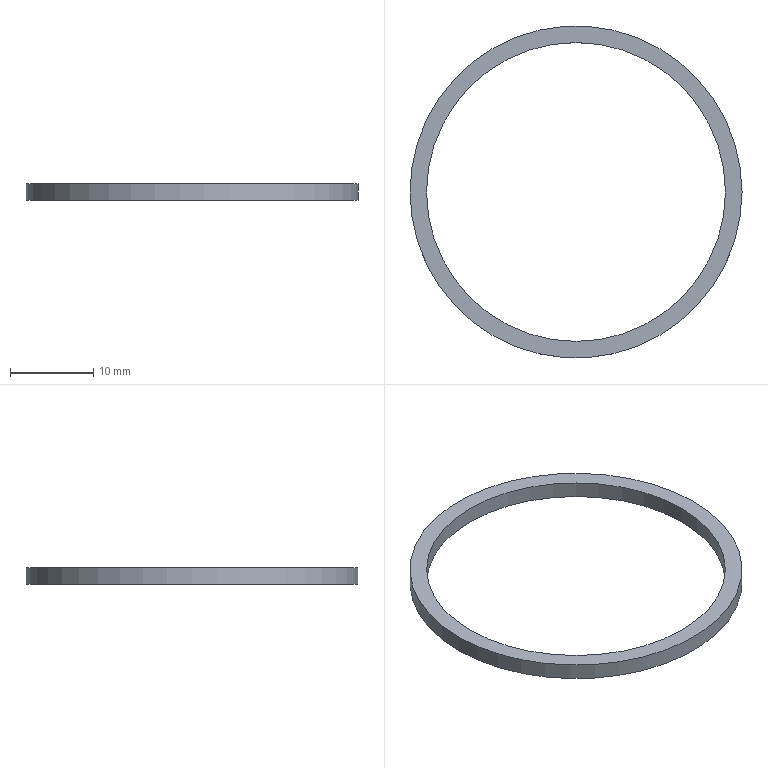Part | NX | features DATUM_CSYS 2, EXTRUDE 1, SKETCH 1 | 1 solid | 4 faces | box 40 x 40 x 2 mm | volume 477.522 mm3 | cylinder 2 | plane 2 | commonest cylinder face diameters 36 x1 40 x1
STEP:
#1=CARTESIAN_POINT('',(20.,0.,2.));
#2=VERTEX_POINT('',#1);
#3=CARTESIAN_POINT('',(0.,0.,2.));
#4=DIRECTION('',(0.,0.,1.));
#5=DIRECTION('',(1.,0.,0.));
#6=AXIS2_PLACEMENT_3D('',#3,#4,#5);
#7=CIRCLE('',#6,20.);
#8=EDGE_CURVE('',#2,#2,#7,.T.);
#9=ORIENTED_EDGE('',*,*,#8,.F.);
#10=EDGE_LOOP('',(#9));
#11=FACE_BOUND('',#10,.T.);
#12=CARTESIAN_POINT('',(20.,0.,0.));
#13=VERTEX_POINT('',#12);
#14=CARTESIAN_POINT('',(0.,0.,0.));
#15=DIRECTION('',(0.,0.,1.));
#16=DIRECTION('',(1.,0.,0.));
#17=AXIS2_PLACEMENT_3D('',#14,#15,#16);
#18=CIRCLE('',#17,20.);
#19=EDGE_CURVE('',#13,#13,#18,.T.);
#20=ORIENTED_EDGE('',*,*,#19,.T.);
#21=EDGE_LOOP('',(#20));
#22=FACE_BOUND('',#21,.T.);
#23=CARTESIAN_POINT('',(0.,0.,2.));
#24=DIRECTION('',(0.,0.,-1.));
#25=DIRECTION('',(-1.,0.,0.));
#26=AXIS2_PLACEMENT_3D('',#23,#24,#25);
#27=CYLINDRICAL_SURFACE('',#26,20.);
#28=ADVANCED_FACE('',(#11,#22),#27,.T.);
#29=CARTESIAN_POINT('',(18.,0.,2.));
#30=VERTEX_POINT('',#29);
#31=CARTESIAN_POINT('',(0.,0.,2.));
#32=DIRECTION('',(0.,0.,1.));
#33=DIRECTION('',(1.,0.,0.));
#34=AXIS2_PLACEMENT_3D('',#31,#32,#33);
#35=CIRCLE('',#34,18.);
#36=EDGE_CURVE('',#30,#30,#35,.T.);
#37=ORIENTED_EDGE('',*,*,#36,.T.);
#38=EDGE_LOOP('',(#37));
#39=FACE_BOUND('',#38,.T.);
#40=CARTESIAN_POINT('',(18.,0.,0.));
#41=VERTEX_POINT('',#40);
#42=CARTESIAN_POINT('',(0.,0.,0.));
#43=DIRECTION('',(0.,0.,1.));
#44=DIRECTION('',(1.,0.,0.));
#45=AXIS2_PLACEMENT_3D('',#42,#43,#44);
#46=CIRCLE('',#45,18.);
#47=EDGE_CURVE('',#41,#41,#46,.T.);
#48=ORIENTED_EDGE('',*,*,#47,.F.);
#49=EDGE_LOOP('',(#48));
#50=FACE_BOUND('',#49,.T.);
#51=CARTESIAN_POINT('',(0.,0.,2.));
#52=DIRECTION('',(0.,0.,-1.));
#53=DIRECTION('',(-1.,0.,0.));
#54=AXIS2_PLACEMENT_3D('',#51,#52,#53);
#55=CYLINDRICAL_SURFACE('',#54,18.);
#56=ADVANCED_FACE('',(#39,#50),#55,.F.);
#57=ORIENTED_EDGE('',*,*,#8,.T.);
#58=EDGE_LOOP('',(#57));
#59=FACE_BOUND('',#58,.T.);
#60=ORIENTED_EDGE('',*,*,#36,.F.);
#61=EDGE_LOOP('',(#60));
#62=FACE_BOUND('',#61,.T.);
#63=CARTESIAN_POINT('',(0.,0.,2.));
#64=DIRECTION('',(0.,0.,1.));
#65=DIRECTION('',(1.,0.,0.));
#66=AXIS2_PLACEMENT_3D('',#63,#64,#65);
#67=PLANE('',#66);
#68=ADVANCED_FACE('',(#59,#62),#67,.T.);
#69=ORIENTED_EDGE('',*,*,#19,.F.);
#70=EDGE_LOOP('',(#69));
#71=FACE_BOUND('',#70,.T.);
#72=ORIENTED_EDGE('',*,*,#47,.T.);
#73=EDGE_LOOP('',(#72));
#74=FACE_BOUND('',#73,.T.);
#75=CARTESIAN_POINT('',(0.,0.,0.));
#76=DIRECTION('',(0.,0.,1.));
#77=DIRECTION('',(1.,0.,0.));
#78=AXIS2_PLACEMENT_3D('',#75,#76,#77);
#79=PLANE('',#78);
#80=ADVANCED_FACE('',(#71,#74),#79,.F.);
#81=CLOSED_SHELL('',(#28,#56,#68,#80));
#82=MANIFOLD_SOLID_BREP('',#81);
#83=(LENGTH_UNIT()NAMED_UNIT(*)SI_UNIT(.MILLI.,.METRE.));
#84=UNCERTAINTY_MEASURE_WITH_UNIT(LENGTH_MEASURE(0.00001),#83,'','');
#85=(NAMED_UNIT(*)PLANE_ANGLE_UNIT()SI_UNIT($,.RADIAN.));
#86=(NAMED_UNIT(*)SI_UNIT($,.STERADIAN.)SOLID_ANGLE_UNIT());
#87=(GEOMETRIC_REPRESENTATION_CONTEXT(3)GLOBAL_UNCERTAINTY_ASSIGNED_CONTEXT((#84))GLOBAL_UNIT_ASSIGNED_CONTEXT((#83,#85,#86))REPRESENTATION_CONTEXT('',''));
#88=ADVANCED_BREP_SHAPE_REPRESENTATION('',(#82),#87);